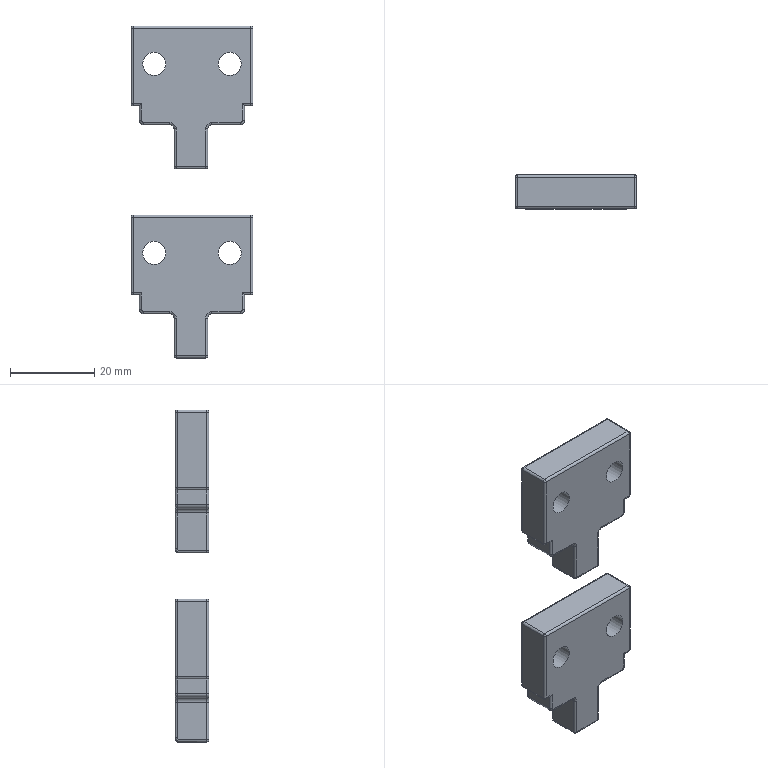Part | 2 solids | 152 faces | box 29 x 8 x 79 mm | volume 11165 mm3 | cylinder 78 | plane 30 | sphere 24 | torus 16 | spline 4 | commonest cylinder face diameters 1 x64 2 x8 5.5 x4 0.4 x2